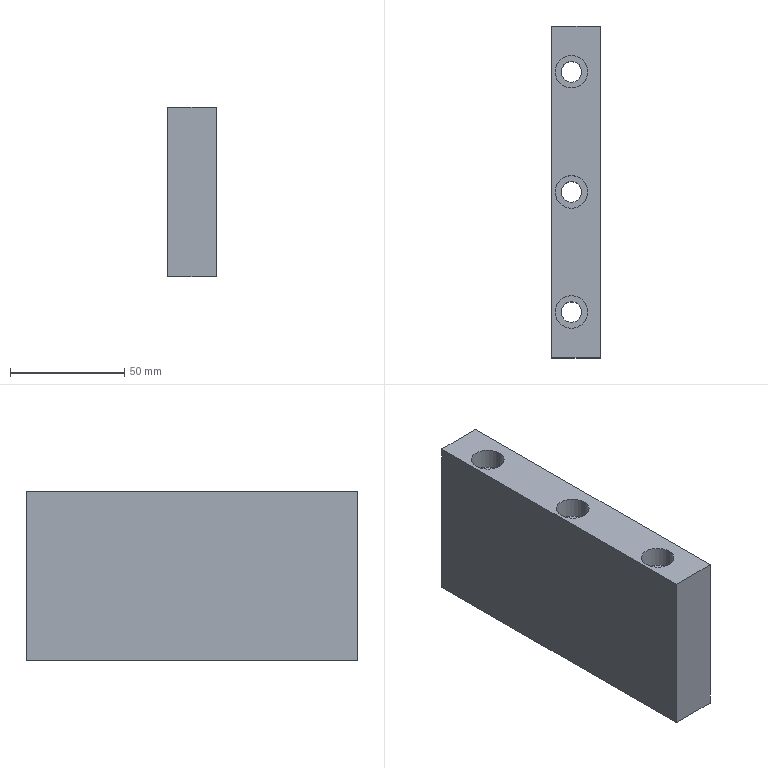Part | Creo | 1 solid | 21 faces | box 21 x 145 x 74 mm | volume 208619 mm3 | cylinder 12 | plane 9 | commonest cylinder face diameters 9 x6 14.25 x6
STEP:
#1=CARTESIAN_POINT('',(0.,0.,0.));
#2=DIRECTION('',(0.,0.,1.));
#3=DIRECTION('',(1.,0.,0.));
#4=AXIS2_PLACEMENT_3D('',#1,#2,#3);
#5=CARTESIAN_POINT('',(-29.668,270.373,-103.441));
#6=VERTEX_POINT('',#5);
#7=CARTESIAN_POINT('',(-29.668,125.373,-103.441));
#8=VERTEX_POINT('',#7);
#9=CARTESIAN_POINT('',(-29.668,270.373,-103.441));
#10=DIRECTION('',(0.000000046,-1.,0.));
#11=VECTOR('',#10,145.);
#12=LINE('',#9,#11);
#13=EDGE_CURVE('',#6,#8,#12,.T.);
#14=ORIENTED_EDGE('',*,*,#13,.F.);
#15=CARTESIAN_POINT('',(-50.668,270.373,-103.441));
#16=VERTEX_POINT('',#15);
#17=CARTESIAN_POINT('',(-29.668,270.373,-103.441));
#18=DIRECTION('',(-1.,0.,0.));
#19=VECTOR('',#18,21.);
#20=LINE('',#17,#19);
#21=EDGE_CURVE('',#6,#16,#20,.T.);
#22=ORIENTED_EDGE('',*,*,#21,.T.);
#23=CARTESIAN_POINT('',(-50.668,125.373,-103.441));
#24=VERTEX_POINT('',#23);
#25=CARTESIAN_POINT('',(-50.668,270.373,-103.441));
#26=DIRECTION('',(0.000000046,-1.,0.));
#27=VECTOR('',#26,145.);
#28=LINE('',#25,#27);
#29=EDGE_CURVE('',#16,#24,#28,.T.);
#30=ORIENTED_EDGE('',*,*,#29,.T.);
#31=CARTESIAN_POINT('',(-50.668,125.373,-103.441));
#32=DIRECTION('',(1.,0.,0.));
#33=VECTOR('',#32,21.);
#34=LINE('',#31,#33);
#35=EDGE_CURVE('',#24,#8,#34,.T.);
#36=ORIENTED_EDGE('',*,*,#35,.T.);
#37=EDGE_LOOP('',(#14,#22,#30,#36));
#38=FACE_OUTER_BOUND('',#37,.F.);
#39=CARTESIAN_POINT('',(-46.668,250.373,-103.441));
#40=VERTEX_POINT('',#39);
#41=CARTESIAN_POINT('',(-37.668,250.373,-103.441));
#42=VERTEX_POINT('',#41);
#43=CARTESIAN_POINT('',(-42.168,250.373,-103.441));
#44=DIRECTION('',(0.,0.,1.));
#45=DIRECTION('',(-1.,0.,0.));
#46=AXIS2_PLACEMENT_3D('',#43,#44,#45);
#47=CIRCLE('',#46,4.5);
#48=EDGE_CURVE('',#40,#42,#47,.T.);
#49=ORIENTED_EDGE('',*,*,#48,.F.);
#50=CARTESIAN_POINT('',(-42.168,250.373,-103.441));
#51=DIRECTION('',(0.,0.,1.));
#52=DIRECTION('',(1.,0.,0.));
#53=AXIS2_PLACEMENT_3D('',#50,#51,#52);
#54=CIRCLE('',#53,4.5);
#55=EDGE_CURVE('',#42,#40,#54,.T.);
#56=ORIENTED_EDGE('',*,*,#55,.F.);
#57=EDGE_LOOP('',(#49,#56));
#58=FACE_BOUND('',#57,.F.);
#59=CARTESIAN_POINT('',(-46.668,145.373,-103.441));
#60=VERTEX_POINT('',#59);
#61=CARTESIAN_POINT('',(-37.668,145.373,-103.441));
#62=VERTEX_POINT('',#61);
#63=CARTESIAN_POINT('',(-42.168,145.373,-103.441));
#64=DIRECTION('',(0.,0.,1.));
#65=DIRECTION('',(-1.,0.,0.));
#66=AXIS2_PLACEMENT_3D('',#63,#64,#65);
#67=CIRCLE('',#66,4.5);
#68=EDGE_CURVE('',#60,#62,#67,.T.);
#69=ORIENTED_EDGE('',*,*,#68,.F.);
#70=CARTESIAN_POINT('',(-42.168,145.373,-103.441));
#71=DIRECTION('',(0.,0.,1.));
#72=DIRECTION('',(1.,0.,0.));
#73=AXIS2_PLACEMENT_3D('',#70,#71,#72);
#74=CIRCLE('',#73,4.5);
#75=EDGE_CURVE('',#62,#60,#74,.T.);
#76=ORIENTED_EDGE('',*,*,#75,.F.);
#77=EDGE_LOOP('',(#69,#76));
#78=FACE_BOUND('',#77,.F.);
#79=CARTESIAN_POINT('',(-46.668,197.873,-103.441));
#80=VERTEX_POINT('',#79);
#81=CARTESIAN_POINT('',(-37.668,197.873,-103.441));
#82=VERTEX_POINT('',#81);
#83=CARTESIAN_POINT('',(-42.168,197.873,-103.441));
#84=DIRECTION('',(0.,0.,1.));
#85=DIRECTION('',(-1.,0.,0.));
#86=AXIS2_PLACEMENT_3D('',#83,#84,#85);
#87=CIRCLE('',#86,4.5);
#88=EDGE_CURVE('',#80,#82,#87,.T.);
#89=ORIENTED_EDGE('',*,*,#88,.F.);
#90=CARTESIAN_POINT('',(-42.168,197.873,-103.441));
#91=DIRECTION('',(0.,0.,1.));
#92=DIRECTION('',(1.,0.,0.));
#93=AXIS2_PLACEMENT_3D('',#90,#91,#92);
#94=CIRCLE('',#93,4.5);
#95=EDGE_CURVE('',#82,#80,#94,.T.);
#96=ORIENTED_EDGE('',*,*,#95,.F.);
#97=EDGE_LOOP('',(#89,#96));
#98=FACE_BOUND('',#97,.F.);
#99=CARTESIAN_POINT('',(-29.668,140.373,-103.441));
#100=DIRECTION('',(0.,0.,1.));
#101=DIRECTION('',(1.,0.,0.));
#102=AXIS2_PLACEMENT_3D('',#99,#100,#101);
#103=PLANE('',#102);
#104=ADVANCED_FACE('',(#38,#58,#78,#98),#103,.F.);
#105=ORIENTED_EDGE('',*,*,#13,.T.);
#106=CARTESIAN_POINT('',(-29.668,125.373,-29.441));
#107=VERTEX_POINT('',#106);
#108=CARTESIAN_POINT('',(-29.668,125.373,-103.441));
#109=DIRECTION('',(0.,0.,1.));
#110=VECTOR('',#109,74.);
#111=LINE('',#108,#110);
#112=EDGE_CURVE('',#8,#107,#111,.T.);
#113=ORIENTED_EDGE('',*,*,#112,.T.);
#114=CARTESIAN_POINT('',(-29.668,270.373,-29.441));
#115=VERTEX_POINT('',#114);
#116=CARTESIAN_POINT('',(-29.668,270.373,-29.441));
#117=DIRECTION('',(0.000000046,-1.,0.));
#118=VECTOR('',#117,145.);
#119=LINE('',#116,#118);
#120=EDGE_CURVE('',#115,#107,#119,.T.);
#121=ORIENTED_EDGE('',*,*,#120,.F.);
#122=CARTESIAN_POINT('',(-29.668,270.373,-103.441));
#123=DIRECTION('',(0.,0.,1.));
#124=VECTOR('',#123,74.);
#125=LINE('',#122,#124);
#126=EDGE_CURVE('',#6,#115,#125,.T.);
#127=ORIENTED_EDGE('',*,*,#126,.F.);
#128=EDGE_LOOP('',(#105,#113,#121,#127));
#129=FACE_OUTER_BOUND('',#128,.F.);
#130=CARTESIAN_POINT('',(-29.668,23.699,-58.441));
#131=DIRECTION('',(1.,0.000000046,0.));
#132=DIRECTION('',(-0.000000046,1.,0.));
#133=AXIS2_PLACEMENT_3D('',#130,#131,#132);
#134=PLANE('',#133);
#135=ADVANCED_FACE('',(#129),#134,.T.);
#136=ORIENTED_EDGE('',*,*,#35,.F.);
#137=CARTESIAN_POINT('',(-50.668,125.373,-29.441));
#138=VERTEX_POINT('',#137);
#139=CARTESIAN_POINT('',(-50.668,125.373,-103.441));
#140=DIRECTION('',(0.,0.,1.));
#141=VECTOR('',#140,74.);
#142=LINE('',#139,#141);
#143=EDGE_CURVE('',#24,#138,#142,.T.);
#144=ORIENTED_EDGE('',*,*,#143,.T.);
#145=CARTESIAN_POINT('',(-50.668,125.373,-29.441));
#146=DIRECTION('',(1.,0.,0.));
#147=VECTOR('',#146,21.);
#148=LINE('',#145,#147);
#149=EDGE_CURVE('',#138,#107,#148,.T.);
#150=ORIENTED_EDGE('',*,*,#149,.T.);
#151=ORIENTED_EDGE('',*,*,#112,.F.);
#152=EDGE_LOOP('',(#136,#144,#150,#151));
#153=FACE_OUTER_BOUND('',#152,.F.);
#154=CARTESIAN_POINT('',(64.101,125.373,-27.043));
#155=DIRECTION('',(0.,1.,0.));
#156=DIRECTION('',(0.,0.,1.));
#157=AXIS2_PLACEMENT_3D('',#154,#155,#156);
#158=PLANE('',#157);
#159=ADVANCED_FACE('',(#153),#158,.F.);
#160=ORIENTED_EDGE('',*,*,#29,.F.);
#161=CARTESIAN_POINT('',(-50.668,270.373,-29.441));
#162=VERTEX_POINT('',#161);
#163=CARTESIAN_POINT('',(-50.668,270.373,-103.441));
#164=DIRECTION('',(0.,0.,1.));
#165=VECTOR('',#164,74.);
#166=LINE('',#163,#165);
#167=EDGE_CURVE('',#16,#162,#166,.T.);
#168=ORIENTED_EDGE('',*,*,#167,.T.);
#169=CARTESIAN_POINT('',(-50.668,270.373,-29.441));
#170=DIRECTION('',(0.000000046,-1.,0.));
#171=VECTOR('',#170,145.);
#172=LINE('',#169,#171);
#173=EDGE_CURVE('',#162,#138,#172,.T.);
#174=ORIENTED_EDGE('',*,*,#173,.T.);
#175=ORIENTED_EDGE('',*,*,#143,.F.);
#176=EDGE_LOOP('',(#160,#168,#174,#175));
#177=FACE_OUTER_BOUND('',#176,.F.);
#178=CARTESIAN_POINT('',(-50.668,140.373,-58.441));
#179=DIRECTION('',(1.,0.000000046,0.));
#180=DIRECTION('',(-0.000000046,1.,0.));
#181=AXIS2_PLACEMENT_3D('',#178,#179,#180);
#182=PLANE('',#181);
#183=ADVANCED_FACE('',(#177),#182,.F.);
#184=ORIENTED_EDGE('',*,*,#21,.F.);
#185=ORIENTED_EDGE('',*,*,#126,.T.);
#186=CARTESIAN_POINT('',(-29.668,270.373,-29.441));
#187=DIRECTION('',(-1.,0.,0.));
#188=VECTOR('',#187,21.);
#189=LINE('',#186,#188);
#190=EDGE_CURVE('',#115,#162,#189,.T.);
#191=ORIENTED_EDGE('',*,*,#190,.T.);
#192=ORIENTED_EDGE('',*,*,#167,.F.);
#193=EDGE_LOOP('',(#184,#185,#191,#192));
#194=FACE_OUTER_BOUND('',#193,.F.);
#195=CARTESIAN_POINT('',(-335.899,270.373,-228.441));
#196=DIRECTION('',(0.,-1.,0.));
#197=DIRECTION('',(1.,0.,0.));
#198=AXIS2_PLACEMENT_3D('',#195,#196,#197);
#199=PLANE('',#198);
#200=ADVANCED_FACE('',(#194),#199,.F.);
#201=ORIENTED_EDGE('',*,*,#120,.T.);
#202=ORIENTED_EDGE('',*,*,#149,.F.);
#203=ORIENTED_EDGE('',*,*,#173,.F.);
#204=ORIENTED_EDGE('',*,*,#190,.F.);
#205=EDGE_LOOP('',(#201,#202,#203,#204));
#206=FACE_OUTER_BOUND('',#205,.F.);
#207=CARTESIAN_POINT('',(-35.043,145.373,-29.441));
#208=VERTEX_POINT('',#207);
#209=CARTESIAN_POINT('',(-49.293,145.373,-29.441));
#210=VERTEX_POINT('',#209);
#211=CARTESIAN_POINT('',(-42.168,145.373,-29.441));
#212=DIRECTION('',(0.,0.,-1.));
#213=DIRECTION('',(1.,0.,0.));
#214=AXIS2_PLACEMENT_3D('',#211,#212,#213);
#215=CIRCLE('',#214,7.125);
#216=EDGE_CURVE('',#208,#210,#215,.T.);
#217=ORIENTED_EDGE('',*,*,#216,.F.);
#218=CARTESIAN_POINT('',(-42.168,145.373,-29.441));
#219=DIRECTION('',(0.,0.,-1.));
#220=DIRECTION('',(-1.,0.,0.));
#221=AXIS2_PLACEMENT_3D('',#218,#219,#220);
#222=CIRCLE('',#221,7.125);
#223=EDGE_CURVE('',#210,#208,#222,.T.);
#224=ORIENTED_EDGE('',*,*,#223,.F.);
#225=EDGE_LOOP('',(#217,#224));
#226=FACE_BOUND('',#225,.F.);
#227=CARTESIAN_POINT('',(-35.043,250.373,-29.441));
#228=VERTEX_POINT('',#227);
#229=CARTESIAN_POINT('',(-49.293,250.373,-29.441));
#230=VERTEX_POINT('',#229);
#231=CARTESIAN_POINT('',(-42.168,250.373,-29.441));
#232=DIRECTION('',(0.,0.,-1.));
#233=DIRECTION('',(1.,0.,0.));
#234=AXIS2_PLACEMENT_3D('',#231,#232,#233);
#235=CIRCLE('',#234,7.125);
#236=EDGE_CURVE('',#228,#230,#235,.T.);
#237=ORIENTED_EDGE('',*,*,#236,.F.);
#238=CARTESIAN_POINT('',(-42.168,250.373,-29.441));
#239=DIRECTION('',(0.,0.,-1.));
#240=DIRECTION('',(-1.,0.,0.));
#241=AXIS2_PLACEMENT_3D('',#238,#239,#240);
#242=CIRCLE('',#241,7.125);
#243=EDGE_CURVE('',#230,#228,#242,.T.);
#244=ORIENTED_EDGE('',*,*,#243,.F.);
#245=EDGE_LOOP('',(#237,#244));
#246=FACE_BOUND('',#245,.F.);
#247=CARTESIAN_POINT('',(-35.043,197.873,-29.441));
#248=VERTEX_POINT('',#247);
#249=CARTESIAN_POINT('',(-49.293,197.873,-29.441));
#250=VERTEX_POINT('',#249);
#251=CARTESIAN_POINT('',(-42.168,197.873,-29.441));
#252=DIRECTION('',(0.,0.,-1.));
#253=DIRECTION('',(1.,0.,0.));
#254=AXIS2_PLACEMENT_3D('',#251,#252,#253);
#255=CIRCLE('',#254,7.125);
#256=EDGE_CURVE('',#248,#250,#255,.T.);
#257=ORIENTED_EDGE('',*,*,#256,.F.);
#258=CARTESIAN_POINT('',(-42.168,197.873,-29.441));
#259=DIRECTION('',(0.,0.,-1.));
#260=DIRECTION('',(-1.,0.,0.));
#261=AXIS2_PLACEMENT_3D('',#258,#259,#260);
#262=CIRCLE('',#261,7.125);
#263=EDGE_CURVE('',#250,#248,#262,.T.);
#264=ORIENTED_EDGE('',*,*,#263,.F.);
#265=EDGE_LOOP('',(#257,#264));
#266=FACE_BOUND('',#265,.F.);
#267=CARTESIAN_POINT('',(-29.668,140.373,-29.441));
#268=DIRECTION('',(0.,0.,1.));
#269=DIRECTION('',(1.,0.,0.));
#270=AXIS2_PLACEMENT_3D('',#267,#268,#269);
#271=PLANE('',#270);
#272=ADVANCED_FACE('',(#206,#226,#246,#266),#271,.T.);
#273=ORIENTED_EDGE('',*,*,#256,.T.);
#274=CARTESIAN_POINT('',(-49.293,197.873,-38.441));
#275=VERTEX_POINT('',#274);
#276=CARTESIAN_POINT('',(-49.293,197.873,-38.441));
#277=DIRECTION('',(0.,0.,1.));
#278=VECTOR('',#277,9.);
#279=LINE('',#276,#278);
#280=EDGE_CURVE('',#275,#250,#279,.T.);
#281=ORIENTED_EDGE('',*,*,#280,.F.);
#282=CARTESIAN_POINT('',(-35.043,197.873,-38.441));
#283=VERTEX_POINT('',#282);
#284=CARTESIAN_POINT('',(-42.168,197.873,-38.441));
#285=DIRECTION('',(0.,0.,1.));
#286=DIRECTION('',(-1.,0.,0.));
#287=AXIS2_PLACEMENT_3D('',#284,#285,#286);
#288=CIRCLE('',#287,7.125);
#289=EDGE_CURVE('',#275,#283,#288,.T.);
#290=ORIENTED_EDGE('',*,*,#289,.T.);
#291=CARTESIAN_POINT('',(-35.043,197.873,-38.441));
#292=DIRECTION('',(0.,0.,1.));
#293=VECTOR('',#292,9.);
#294=LINE('',#291,#293);
#295=EDGE_CURVE('',#283,#248,#294,.T.);
#296=ORIENTED_EDGE('',*,*,#295,.T.);
#297=EDGE_LOOP('',(#273,#281,#290,#296));
#298=FACE_OUTER_BOUND('',#297,.F.);
#299=CARTESIAN_POINT('',(-42.168,197.873,-38.441));
#300=DIRECTION('',(0.,0.,1.));
#301=DIRECTION('',(1.,0.,0.));
#302=AXIS2_PLACEMENT_3D('',#299,#300,#301);
#303=CYLINDRICAL_SURFACE('',#302,7.125);
#304=ADVANCED_FACE('',(#298),#303,.F.);
#305=ORIENTED_EDGE('',*,*,#263,.T.);
#306=ORIENTED_EDGE('',*,*,#295,.F.);
#307=CARTESIAN_POINT('',(-42.168,197.873,-38.441));
#308=DIRECTION('',(0.,0.,1.));
#309=DIRECTION('',(1.,0.,0.));
#310=AXIS2_PLACEMENT_3D('',#307,#308,#309);
#311=CIRCLE('',#310,7.125);
#312=EDGE_CURVE('',#283,#275,#311,.T.);
#313=ORIENTED_EDGE('',*,*,#312,.T.);
#314=ORIENTED_EDGE('',*,*,#280,.T.);
#315=EDGE_LOOP('',(#305,#306,#313,#314));
#316=FACE_OUTER_BOUND('',#315,.F.);
#317=CARTESIAN_POINT('',(-42.168,197.873,-38.441));
#318=DIRECTION('',(0.,0.,1.));
#319=DIRECTION('',(1.,0.,0.));
#320=AXIS2_PLACEMENT_3D('',#317,#318,#319);
#321=CYLINDRICAL_SURFACE('',#320,7.125);
#322=ADVANCED_FACE('',(#316),#321,.F.);
#323=ORIENTED_EDGE('',*,*,#312,.F.);
#324=ORIENTED_EDGE('',*,*,#289,.F.);
#325=EDGE_LOOP('',(#323,#324));
#326=FACE_OUTER_BOUND('',#325,.F.);
#327=CARTESIAN_POINT('',(-46.668,197.873,-38.441));
#328=VERTEX_POINT('',#327);
#329=CARTESIAN_POINT('',(-37.668,197.873,-38.441));
#330=VERTEX_POINT('',#329);
#331=CARTESIAN_POINT('',(-42.168,197.873,-38.441));
#332=DIRECTION('',(0.,0.,-1.));
#333=DIRECTION('',(-1.,0.,0.));
#334=AXIS2_PLACEMENT_3D('',#331,#332,#333);
#335=CIRCLE('',#334,4.5);
#336=EDGE_CURVE('',#328,#330,#335,.T.);
#337=ORIENTED_EDGE('',*,*,#336,.F.);
#338=CARTESIAN_POINT('',(-42.168,197.873,-38.441));
#339=DIRECTION('',(0.,0.,-1.));
#340=DIRECTION('',(1.,0.,0.));
#341=AXIS2_PLACEMENT_3D('',#338,#339,#340);
#342=CIRCLE('',#341,4.5);
#343=EDGE_CURVE('',#330,#328,#342,.T.);
#344=ORIENTED_EDGE('',*,*,#343,.F.);
#345=EDGE_LOOP('',(#337,#344));
#346=FACE_BOUND('',#345,.F.);
#347=CARTESIAN_POINT('',(-42.168,197.873,-38.441));
#348=DIRECTION('',(0.,0.,-1.));
#349=DIRECTION('',(-1.,0.,0.));
#350=AXIS2_PLACEMENT_3D('',#347,#348,#349);
#351=PLANE('',#350);
#352=ADVANCED_FACE('',(#326,#346),#351,.F.);
#353=ORIENTED_EDGE('',*,*,#95,.T.);
#354=CARTESIAN_POINT('',(-46.668,197.873,-38.441));
#355=DIRECTION('',(0.,0.,-1.));
#356=VECTOR('',#355,65.);
#357=LINE('',#354,#356);
#358=EDGE_CURVE('',#328,#80,#357,.T.);
#359=ORIENTED_EDGE('',*,*,#358,.F.);
#360=ORIENTED_EDGE('',*,*,#336,.T.);
#361=CARTESIAN_POINT('',(-37.668,197.873,-38.441));
#362=DIRECTION('',(0.,0.,-1.));
#363=VECTOR('',#362,65.);
#364=LINE('',#361,#363);
#365=EDGE_CURVE('',#330,#82,#364,.T.);
#366=ORIENTED_EDGE('',*,*,#365,.T.);
#367=EDGE_LOOP('',(#353,#359,#360,#366));
#368=FACE_OUTER_BOUND('',#367,.F.);
#369=CARTESIAN_POINT('',(-42.168,197.873,-38.441));
#370=DIRECTION('',(0.,0.,-1.));
#371=DIRECTION('',(-1.,0.,0.));
#372=AXIS2_PLACEMENT_3D('',#369,#370,#371);
#373=CYLINDRICAL_SURFACE('',#372,4.5);
#374=ADVANCED_FACE('',(#368),#373,.F.);
#375=ORIENTED_EDGE('',*,*,#88,.T.);
#376=ORIENTED_EDGE('',*,*,#365,.F.);
#377=ORIENTED_EDGE('',*,*,#343,.T.);
#378=ORIENTED_EDGE('',*,*,#358,.T.);
#379=EDGE_LOOP('',(#375,#376,#377,#378));
#380=FACE_OUTER_BOUND('',#379,.F.);
#381=CARTESIAN_POINT('',(-42.168,197.873,-38.441));
#382=DIRECTION('',(0.,0.,-1.));
#383=DIRECTION('',(-1.,0.,0.));
#384=AXIS2_PLACEMENT_3D('',#381,#382,#383);
#385=CYLINDRICAL_SURFACE('',#384,4.5);
#386=ADVANCED_FACE('',(#380),#385,.F.);
#387=ORIENTED_EDGE('',*,*,#216,.T.);
#388=CARTESIAN_POINT('',(-49.293,145.373,-38.441));
#389=VERTEX_POINT('',#388);
#390=CARTESIAN_POINT('',(-49.293,145.373,-38.441));
#391=DIRECTION('',(0.,0.,1.));
#392=VECTOR('',#391,9.);
#393=LINE('',#390,#392);
#394=EDGE_CURVE('',#389,#210,#393,.T.);
#395=ORIENTED_EDGE('',*,*,#394,.F.);
#396=CARTESIAN_POINT('',(-35.043,145.373,-38.441));
#397=VERTEX_POINT('',#396);
#398=CARTESIAN_POINT('',(-42.168,145.373,-38.441));
#399=DIRECTION('',(0.,0.,1.));
#400=DIRECTION('',(-1.,0.,0.));
#401=AXIS2_PLACEMENT_3D('',#398,#399,#400);
#402=CIRCLE('',#401,7.125);
#403=EDGE_CURVE('',#389,#397,#402,.T.);
#404=ORIENTED_EDGE('',*,*,#403,.T.);
#405=CARTESIAN_POINT('',(-35.043,145.373,-38.441));
#406=DIRECTION('',(0.,0.,1.));
#407=VECTOR('',#406,9.);
#408=LINE('',#405,#407);
#409=EDGE_CURVE('',#397,#208,#408,.T.);
#410=ORIENTED_EDGE('',*,*,#409,.T.);
#411=EDGE_LOOP('',(#387,#395,#404,#410));
#412=FACE_OUTER_BOUND('',#411,.F.);
#413=CARTESIAN_POINT('',(-42.168,145.373,-38.441));
#414=DIRECTION('',(0.,0.,1.));
#415=DIRECTION('',(1.,0.,0.));
#416=AXIS2_PLACEMENT_3D('',#413,#414,#415);
#417=CYLINDRICAL_SURFACE('',#416,7.125);
#418=ADVANCED_FACE('',(#412),#417,.F.);
#419=ORIENTED_EDGE('',*,*,#223,.T.);
#420=ORIENTED_EDGE('',*,*,#409,.F.);
#421=CARTESIAN_POINT('',(-42.168,145.373,-38.441));
#422=DIRECTION('',(0.,0.,1.));
#423=DIRECTION('',(1.,0.,0.));
#424=AXIS2_PLACEMENT_3D('',#421,#422,#423);
#425=CIRCLE('',#424,7.125);
#426=EDGE_CURVE('',#397,#389,#425,.T.);
#427=ORIENTED_EDGE('',*,*,#426,.T.);
#428=ORIENTED_EDGE('',*,*,#394,.T.);
#429=EDGE_LOOP('',(#419,#420,#427,#428));
#430=FACE_OUTER_BOUND('',#429,.F.);
#431=CARTESIAN_POINT('',(-42.168,145.373,-38.441));
#432=DIRECTION('',(0.,0.,1.));
#433=DIRECTION('',(1.,0.,0.));
#434=AXIS2_PLACEMENT_3D('',#431,#432,#433);
#435=CYLINDRICAL_SURFACE('',#434,7.125);
#436=ADVANCED_FACE('',(#430),#435,.F.);
#437=ORIENTED_EDGE('',*,*,#426,.F.);
#438=ORIENTED_EDGE('',*,*,#403,.F.);
#439=EDGE_LOOP('',(#437,#438));
#440=FACE_OUTER_BOUND('',#439,.F.);
#441=CARTESIAN_POINT('',(-46.668,145.373,-38.441));
#442=VERTEX_POINT('',#441);
#443=CARTESIAN_POINT('',(-37.668,145.373,-38.441));
#444=VERTEX_POINT('',#443);
#445=CARTESIAN_POINT('',(-42.168,145.373,-38.441));
#446=DIRECTION('',(0.,0.,-1.));
#447=DIRECTION('',(-1.,0.,0.));
#448=AXIS2_PLACEMENT_3D('',#445,#446,#447);
#449=CIRCLE('',#448,4.5);
#450=EDGE_CURVE('',#442,#444,#449,.T.);
#451=ORIENTED_EDGE('',*,*,#450,.F.);
#452=CARTESIAN_POINT('',(-42.168,145.373,-38.441));
#453=DIRECTION('',(0.,0.,-1.));
#454=DIRECTION('',(1.,0.,0.));
#455=AXIS2_PLACEMENT_3D('',#452,#453,#454);
#456=CIRCLE('',#455,4.5);
#457=EDGE_CURVE('',#444,#442,#456,.T.);
#458=ORIENTED_EDGE('',*,*,#457,.F.);
#459=EDGE_LOOP('',(#451,#458));
#460=FACE_BOUND('',#459,.F.);
#461=CARTESIAN_POINT('',(-42.168,145.373,-38.441));
#462=DIRECTION('',(0.,0.,-1.));
#463=DIRECTION('',(-1.,0.,0.));
#464=AXIS2_PLACEMENT_3D('',#461,#462,#463);
#465=PLANE('',#464);
#466=ADVANCED_FACE('',(#440,#460),#465,.F.);
#467=ORIENTED_EDGE('',*,*,#75,.T.);
#468=CARTESIAN_POINT('',(-46.668,145.373,-38.441));
#469=DIRECTION('',(0.,0.,-1.));
#470=VECTOR('',#469,65.);
#471=LINE('',#468,#470);
#472=EDGE_CURVE('',#442,#60,#471,.T.);
#473=ORIENTED_EDGE('',*,*,#472,.F.);
#474=ORIENTED_EDGE('',*,*,#450,.T.);
#475=CARTESIAN_POINT('',(-37.668,145.373,-38.441));
#476=DIRECTION('',(0.,0.,-1.));
#477=VECTOR('',#476,65.);
#478=LINE('',#475,#477);
#479=EDGE_CURVE('',#444,#62,#478,.T.);
#480=ORIENTED_EDGE('',*,*,#479,.T.);
#481=EDGE_LOOP('',(#467,#473,#474,#480));
#482=FACE_OUTER_BOUND('',#481,.F.);
#483=CARTESIAN_POINT('',(-42.168,145.373,-38.441));
#484=DIRECTION('',(0.,0.,-1.));
#485=DIRECTION('',(-1.,0.,0.));
#486=AXIS2_PLACEMENT_3D('',#483,#484,#485);
#487=CYLINDRICAL_SURFACE('',#486,4.5);
#488=ADVANCED_FACE('',(#482),#487,.F.);
#489=ORIENTED_EDGE('',*,*,#68,.T.);
#490=ORIENTED_EDGE('',*,*,#479,.F.);
#491=ORIENTED_EDGE('',*,*,#457,.T.);
#492=ORIENTED_EDGE('',*,*,#472,.T.);
#493=EDGE_LOOP('',(#489,#490,#491,#492));
#494=FACE_OUTER_BOUND('',#493,.F.);
#495=CARTESIAN_POINT('',(-42.168,145.373,-38.441));
#496=DIRECTION('',(0.,0.,-1.));
#497=DIRECTION('',(-1.,0.,0.));
#498=AXIS2_PLACEMENT_3D('',#495,#496,#497);
#499=CYLINDRICAL_SURFACE('',#498,4.5);
#500=ADVANCED_FACE('',(#494),#499,.F.);
#501=ORIENTED_EDGE('',*,*,#236,.T.);
#502=CARTESIAN_POINT('',(-49.293,250.373,-38.441));
#503=VERTEX_POINT('',#502);
#504=CARTESIAN_POINT('',(-49.293,250.373,-38.441));
#505=DIRECTION('',(0.,0.,1.));
#506=VECTOR('',#505,9.);
#507=LINE('',#504,#506);
#508=EDGE_CURVE('',#503,#230,#507,.T.);
#509=ORIENTED_EDGE('',*,*,#508,.F.);
#510=CARTESIAN_POINT('',(-35.043,250.373,-38.441));
#511=VERTEX_POINT('',#510);
#512=CARTESIAN_POINT('',(-42.168,250.373,-38.441));
#513=DIRECTION('',(0.,0.,1.));
#514=DIRECTION('',(-1.,0.,0.));
#515=AXIS2_PLACEMENT_3D('',#512,#513,#514);
#516=CIRCLE('',#515,7.125);
#517=EDGE_CURVE('',#503,#511,#516,.T.);
#518=ORIENTED_EDGE('',*,*,#517,.T.);
#519=CARTESIAN_POINT('',(-35.043,250.373,-38.441));
#520=DIRECTION('',(0.,0.,1.));
#521=VECTOR('',#520,9.);
#522=LINE('',#519,#521);
#523=EDGE_CURVE('',#511,#228,#522,.T.);
#524=ORIENTED_EDGE('',*,*,#523,.T.);
#525=EDGE_LOOP('',(#501,#509,#518,#524));
#526=FACE_OUTER_BOUND('',#525,.F.);
#527=CARTESIAN_POINT('',(-42.168,250.373,-38.441));
#528=DIRECTION('',(0.,0.,1.));
#529=DIRECTION('',(1.,0.,0.));
#530=AXIS2_PLACEMENT_3D('',#527,#528,#529);
#531=CYLINDRICAL_SURFACE('',#530,7.125);
#532=ADVANCED_FACE('',(#526),#531,.F.);
#533=ORIENTED_EDGE('',*,*,#243,.T.);
#534=ORIENTED_EDGE('',*,*,#523,.F.);
#535=CARTESIAN_POINT('',(-42.168,250.373,-38.441));
#536=DIRECTION('',(0.,0.,1.));
#537=DIRECTION('',(1.,0.,0.));
#538=AXIS2_PLACEMENT_3D('',#535,#536,#537);
#539=CIRCLE('',#538,7.125);
#540=EDGE_CURVE('',#511,#503,#539,.T.);
#541=ORIENTED_EDGE('',*,*,#540,.T.);
#542=ORIENTED_EDGE('',*,*,#508,.T.);
#543=EDGE_LOOP('',(#533,#534,#541,#542));
#544=FACE_OUTER_BOUND('',#543,.F.);
#545=CARTESIAN_POINT('',(-42.168,250.373,-38.441));
#546=DIRECTION('',(0.,0.,1.));
#547=DIRECTION('',(1.,0.,0.));
#548=AXIS2_PLACEMENT_3D('',#545,#546,#547);
#549=CYLINDRICAL_SURFACE('',#548,7.125);
#550=ADVANCED_FACE('',(#544),#549,.F.);
#551=ORIENTED_EDGE('',*,*,#540,.F.);
#552=ORIENTED_EDGE('',*,*,#517,.F.);
#553=EDGE_LOOP('',(#551,#552));
#554=FACE_OUTER_BOUND('',#553,.F.);
#555=CARTESIAN_POINT('',(-46.668,250.373,-38.441));
#556=VERTEX_POINT('',#555);
#557=CARTESIAN_POINT('',(-37.668,250.373,-38.441));
#558=VERTEX_POINT('',#557);
#559=CARTESIAN_POINT('',(-42.168,250.373,-38.441));
#560=DIRECTION('',(0.,0.,-1.));
#561=DIRECTION('',(-1.,0.,0.));
#562=AXIS2_PLACEMENT_3D('',#559,#560,#561);
#563=CIRCLE('',#562,4.5);
#564=EDGE_CURVE('',#556,#558,#563,.T.);
#565=ORIENTED_EDGE('',*,*,#564,.F.);
#566=CARTESIAN_POINT('',(-42.168,250.373,-38.441));
#567=DIRECTION('',(0.,0.,-1.));
#568=DIRECTION('',(1.,0.,0.));
#569=AXIS2_PLACEMENT_3D('',#566,#567,#568);
#570=CIRCLE('',#569,4.5);
#571=EDGE_CURVE('',#558,#556,#570,.T.);
#572=ORIENTED_EDGE('',*,*,#571,.F.);
#573=EDGE_LOOP('',(#565,#572));
#574=FACE_BOUND('',#573,.F.);
#575=CARTESIAN_POINT('',(-42.168,250.373,-38.441));
#576=DIRECTION('',(0.,0.,-1.));
#577=DIRECTION('',(-1.,0.,0.));
#578=AXIS2_PLACEMENT_3D('',#575,#576,#577);
#579=PLANE('',#578);
#580=ADVANCED_FACE('',(#554,#574),#579,.F.);
#581=ORIENTED_EDGE('',*,*,#55,.T.);
#582=CARTESIAN_POINT('',(-46.668,250.373,-38.441));
#583=DIRECTION('',(0.,0.,-1.));
#584=VECTOR('',#583,65.);
#585=LINE('',#582,#584);
#586=EDGE_CURVE('',#556,#40,#585,.T.);
#587=ORIENTED_EDGE('',*,*,#586,.F.);
#588=ORIENTED_EDGE('',*,*,#564,.T.);
#589=CARTESIAN_POINT('',(-37.668,250.373,-38.441));
#590=DIRECTION('',(0.,0.,-1.));
#591=VECTOR('',#590,65.);
#592=LINE('',#589,#591);
#593=EDGE_CURVE('',#558,#42,#592,.T.);
#594=ORIENTED_EDGE('',*,*,#593,.T.);
#595=EDGE_LOOP('',(#581,#587,#588,#594));
#596=FACE_OUTER_BOUND('',#595,.F.);
#597=CARTESIAN_POINT('',(-42.168,250.373,-38.441));
#598=DIRECTION('',(0.,0.,-1.));
#599=DIRECTION('',(-1.,0.,0.));
#600=AXIS2_PLACEMENT_3D('',#597,#598,#599);
#601=CYLINDRICAL_SURFACE('',#600,4.5);
#602=ADVANCED_FACE('',(#596),#601,.F.);
#603=ORIENTED_EDGE('',*,*,#48,.T.);
#604=ORIENTED_EDGE('',*,*,#593,.F.);
#605=ORIENTED_EDGE('',*,*,#571,.T.);
#606=ORIENTED_EDGE('',*,*,#586,.T.);
#607=EDGE_LOOP('',(#603,#604,#605,#606));
#608=FACE_OUTER_BOUND('',#607,.F.);
#609=CARTESIAN_POINT('',(-42.168,250.373,-38.441));
#610=DIRECTION('',(0.,0.,-1.));
#611=DIRECTION('',(-1.,0.,0.));
#612=AXIS2_PLACEMENT_3D('',#609,#610,#611);
#613=CYLINDRICAL_SURFACE('',#612,4.5);
#614=ADVANCED_FACE('',(#608),#613,.F.);
#615=CLOSED_SHELL('',(#104,#135,#159,#183,#200,#272,#304,#322,#352,#374,#386,#418,#436,#466,#488,#500,#532,#550,#580,#602,#614));
#616=MANIFOLD_SOLID_BREP('',#615);
#617=(LENGTH_UNIT()NAMED_UNIT(*)SI_UNIT(.MILLI.,.METRE.));
#618=UNCERTAINTY_MEASURE_WITH_UNIT(LENGTH_MEASURE(0.01641),#617,'','');
#619=(NAMED_UNIT(*)PLANE_ANGLE_UNIT()SI_UNIT($,.RADIAN.));
#620=PLANE_ANGLE_MEASURE_WITH_UNIT(PLANE_ANGLE_MEASURE(0.01745),#619);
#621=(CONVERSION_BASED_UNIT('DEGREE',#620)NAMED_UNIT(*)PLANE_ANGLE_UNIT());
#622=(NAMED_UNIT(*)SI_UNIT($,.STERADIAN.)SOLID_ANGLE_UNIT());
#623=(GEOMETRIC_REPRESENTATION_CONTEXT(3)GLOBAL_UNCERTAINTY_ASSIGNED_CONTEXT((#618))GLOBAL_UNIT_ASSIGNED_CONTEXT((#617,#621,#622))REPRESENTATION_CONTEXT('',''));
#624=ADVANCED_BREP_SHAPE_REPRESENTATION('',(#4,#616),#623);